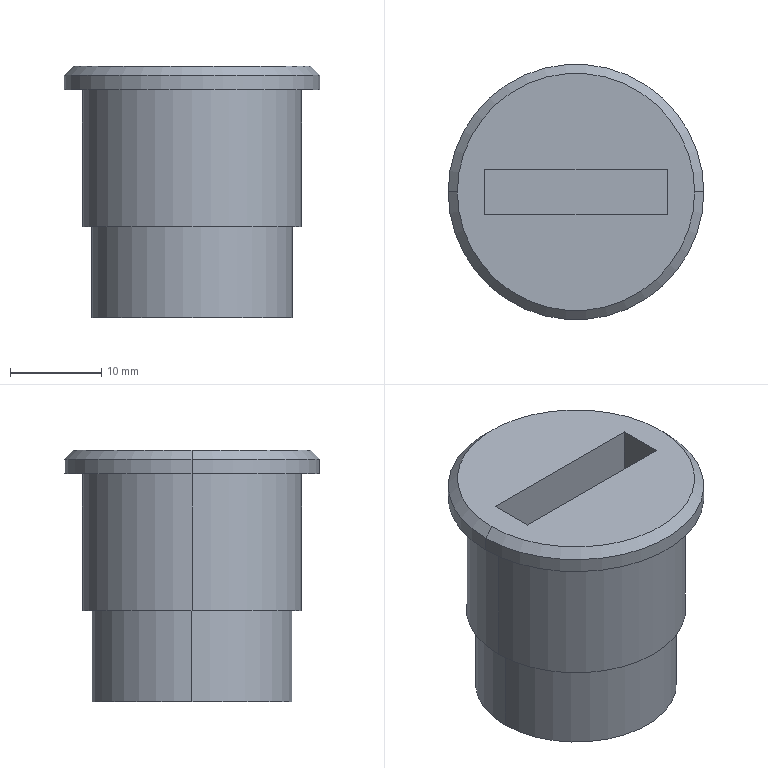Part | STEP file | USB port | 1 solid | 17 faces | box 28 x 28 x 27.6 mm | volume 11145 mm3 | plane 9 | cylinder 6 | cone 2 | commonest cylinder face diameters 22 x2 24 x2 28 x2
STEP:
#1=CARTESIAN_POINT('',(0.,0.,0.));
#2=DIRECTION('',(0.,0.,1.));
#3=DIRECTION('',(1.,0.,0.));
#4=AXIS2_PLACEMENT_3D('',#1,#2,#3);
#5=CARTESIAN_POINT('',(13.,0.,17.6));
#6=VERTEX_POINT('',#5);
#7=CARTESIAN_POINT('',(-13.,0.,17.6));
#8=VERTEX_POINT('',#7);
#9=CARTESIAN_POINT('',(0.,0.,17.6));
#10=DIRECTION('',(0.,0.,1.));
#11=DIRECTION('',(1.,0.,0.));
#12=AXIS2_PLACEMENT_3D('',#9,#10,#11);
#13=CIRCLE('',#12,13.);
#14=CARTESIAN_POINT('',(0.,0.,17.6));
#15=DIRECTION('',(0.,0.,-1.));
#16=DIRECTION('',(-1.,0.,0.));
#17=AXIS2_PLACEMENT_3D('',#14,#15,#16);
#18=CONICAL_SURFACE('',#17,13.,0.7854);
#19=CARTESIAN_POINT('',(3.142,0.));
#20=DIRECTION('',(-1.,0.));
#21=VECTOR('',#20,1.);
#22=LINE('',#19,#21);
#23=(GEOMETRIC_REPRESENTATION_CONTEXT(2)PARAMETRIC_REPRESENTATION_CONTEXT()REPRESENTATION_CONTEXT('',''));
#24=DEFINITIONAL_REPRESENTATION('',(#22),#23);
#25=PCURVE('',#18,#24);
#26=CARTESIAN_POINT('',(0.,0.,17.6));
#27=DIRECTION('',(0.,0.,1.));
#28=DIRECTION('',(1.,0.,0.));
#29=AXIS2_PLACEMENT_3D('',#26,#27,#28);
#30=PLANE('',#29);
#31=CARTESIAN_POINT('',(0.,0.));
#32=DIRECTION('',(1.,0.));
#33=AXIS2_PLACEMENT_2D('',#31,#32);
#34=CIRCLE('',#33,13.);
#35=(GEOMETRIC_REPRESENTATION_CONTEXT(2)PARAMETRIC_REPRESENTATION_CONTEXT()REPRESENTATION_CONTEXT('',''));
#36=DEFINITIONAL_REPRESENTATION('',(#34),#35);
#37=PCURVE('',#30,#36);
#38=SURFACE_CURVE('',#13,(#25,#37),.PCURVE_S1.);
#39=EDGE_CURVE('',#6,#8,#38,.T.);
#40=ORIENTED_EDGE('',*,*,#39,.F.);
#41=CARTESIAN_POINT('',(14.,0.,16.6));
#42=VERTEX_POINT('',#41);
#43=CARTESIAN_POINT('',(13.,0.,17.6));
#44=DIRECTION('',(0.7071,0.,-0.7071));
#45=VECTOR('',#44,1.);
#46=LINE('',#43,#45);
#47=CARTESIAN_POINT('',(3.142,0.));
#48=DIRECTION('',(0.,1.));
#49=VECTOR('',#48,1.);
#50=LINE('',#47,#49);
#51=(GEOMETRIC_REPRESENTATION_CONTEXT(2)PARAMETRIC_REPRESENTATION_CONTEXT()REPRESENTATION_CONTEXT('',''));
#52=DEFINITIONAL_REPRESENTATION('',(#50),#51);
#53=PCURVE('',#18,#52);
#54=CARTESIAN_POINT('',(0.,0.,17.6));
#55=DIRECTION('',(0.,0.,-1.));
#56=DIRECTION('',(-1.,0.,0.));
#57=AXIS2_PLACEMENT_3D('',#54,#55,#56);
#58=CONICAL_SURFACE('',#57,13.,0.7854);
#59=CARTESIAN_POINT('',(3.142,0.));
#60=DIRECTION('',(0.,1.));
#61=VECTOR('',#60,1.);
#62=LINE('',#59,#61);
#63=(GEOMETRIC_REPRESENTATION_CONTEXT(2)PARAMETRIC_REPRESENTATION_CONTEXT()REPRESENTATION_CONTEXT('',''));
#64=DEFINITIONAL_REPRESENTATION('',(#62),#63);
#65=PCURVE('',#58,#64);
#66=SURFACE_CURVE('',#46,(#53,#65),.PCURVE_S1.);
#67=EDGE_CURVE('',#6,#42,#66,.T.);
#68=ORIENTED_EDGE('',*,*,#67,.T.);
#69=CARTESIAN_POINT('',(-14.,0.,16.6));
#70=VERTEX_POINT('',#69);
#71=CARTESIAN_POINT('',(0.,0.,16.6));
#72=DIRECTION('',(0.,0.,-1.));
#73=DIRECTION('',(1.,0.,0.));
#74=AXIS2_PLACEMENT_3D('',#71,#72,#73);
#75=CIRCLE('',#74,14.);
#76=CARTESIAN_POINT('',(-3.142,1.));
#77=DIRECTION('',(1.,0.));
#78=VECTOR('',#77,1.);
#79=LINE('',#76,#78);
#80=(GEOMETRIC_REPRESENTATION_CONTEXT(2)PARAMETRIC_REPRESENTATION_CONTEXT()REPRESENTATION_CONTEXT('',''));
#81=DEFINITIONAL_REPRESENTATION('',(#79),#80);
#82=PCURVE('',#18,#81);
#83=CARTESIAN_POINT('',(0.,0.,17.6));
#84=DIRECTION('',(0.,0.,-1.));
#85=DIRECTION('',(-1.,0.,0.));
#86=AXIS2_PLACEMENT_3D('',#83,#84,#85);
#87=CYLINDRICAL_SURFACE('',#86,14.);
#88=CARTESIAN_POINT('',(-3.142,1.));
#89=DIRECTION('',(1.,0.));
#90=VECTOR('',#89,1.);
#91=LINE('',#88,#90);
#92=(GEOMETRIC_REPRESENTATION_CONTEXT(2)PARAMETRIC_REPRESENTATION_CONTEXT()REPRESENTATION_CONTEXT('',''));
#93=DEFINITIONAL_REPRESENTATION('',(#91),#92);
#94=PCURVE('',#87,#93);
#95=SURFACE_CURVE('',#75,(#82,#94),.PCURVE_S1.);
#96=EDGE_CURVE('',#70,#42,#95,.T.);
#97=ORIENTED_EDGE('',*,*,#96,.F.);
#98=CARTESIAN_POINT('',(-13.,0.,17.6));
#99=DIRECTION('',(-0.7071,0.,-0.7071));
#100=VECTOR('',#99,1.);
#101=LINE('',#98,#100);
#102=CARTESIAN_POINT('',(0.,0.));
#103=DIRECTION('',(0.,1.));
#104=VECTOR('',#103,1.);
#105=LINE('',#102,#104);
#106=(GEOMETRIC_REPRESENTATION_CONTEXT(2)PARAMETRIC_REPRESENTATION_CONTEXT()REPRESENTATION_CONTEXT('',''));
#107=DEFINITIONAL_REPRESENTATION('',(#105),#106);
#108=PCURVE('',#18,#107);
#109=CARTESIAN_POINT('',(6.283,0.));
#110=DIRECTION('',(0.,1.));
#111=VECTOR('',#110,1.);
#112=LINE('',#109,#111);
#113=(GEOMETRIC_REPRESENTATION_CONTEXT(2)PARAMETRIC_REPRESENTATION_CONTEXT()REPRESENTATION_CONTEXT('',''));
#114=DEFINITIONAL_REPRESENTATION('',(#112),#113);
#115=PCURVE('',#58,#114);
#116=SURFACE_CURVE('',#101,(#108,#115),.PCURVE_S1.);
#117=EDGE_CURVE('',#8,#70,#116,.T.);
#118=ORIENTED_EDGE('',*,*,#117,.F.);
#119=EDGE_LOOP('',(#40,#68,#97,#118));
#120=FACE_BOUND('',#119,.T.);
#121=ADVANCED_FACE('',(#120),#18,.T.);
#122=CARTESIAN_POINT('',(-11.,0.,-10.));
#123=VERTEX_POINT('',#122);
#124=CARTESIAN_POINT('',(11.,0.,-10.));
#125=VERTEX_POINT('',#124);
#126=CARTESIAN_POINT('',(0.,0.,-10.));
#127=DIRECTION('',(0.,0.,-1.));
#128=DIRECTION('',(-1.,0.,0.));
#129=AXIS2_PLACEMENT_3D('',#126,#127,#128);
#130=CIRCLE('',#129,11.);
#131=CARTESIAN_POINT('',(0.,0.,-10.));
#132=DIRECTION('',(0.,0.,1.));
#133=DIRECTION('',(1.,0.,0.));
#134=AXIS2_PLACEMENT_3D('',#131,#132,#133);
#135=CYLINDRICAL_SURFACE('',#134,11.);
#136=CARTESIAN_POINT('',(3.142,0.));
#137=DIRECTION('',(-1.,0.));
#138=VECTOR('',#137,1.);
#139=LINE('',#136,#138);
#140=(GEOMETRIC_REPRESENTATION_CONTEXT(2)PARAMETRIC_REPRESENTATION_CONTEXT()REPRESENTATION_CONTEXT('',''));
#141=DEFINITIONAL_REPRESENTATION('',(#139),#140);
#142=PCURVE('',#135,#141);
#143=CARTESIAN_POINT('',(0.,0.,-10.));
#144=DIRECTION('',(0.,0.,-1.));
#145=DIRECTION('',(-1.,0.,0.));
#146=AXIS2_PLACEMENT_3D('',#143,#144,#145);
#147=PLANE('',#146);
#148=CARTESIAN_POINT('',(0.,0.));
#149=DIRECTION('',(1.,0.));
#150=AXIS2_PLACEMENT_2D('',#148,#149);
#151=CIRCLE('',#150,11.);
#152=(GEOMETRIC_REPRESENTATION_CONTEXT(2)PARAMETRIC_REPRESENTATION_CONTEXT()REPRESENTATION_CONTEXT('',''));
#153=DEFINITIONAL_REPRESENTATION('',(#151),#152);
#154=PCURVE('',#147,#153);
#155=SURFACE_CURVE('',#130,(#142,#154),.PCURVE_S1.);
#156=EDGE_CURVE('',#123,#125,#155,.T.);
#157=ORIENTED_EDGE('',*,*,#156,.F.);
#158=CARTESIAN_POINT('',(-11.,0.,0.));
#159=VERTEX_POINT('',#158);
#160=CARTESIAN_POINT('',(-11.,0.,-10.));
#161=DIRECTION('',(0.,0.,1.));
#162=VECTOR('',#161,1.);
#163=LINE('',#160,#162);
#164=CARTESIAN_POINT('',(3.142,0.));
#165=DIRECTION('',(0.,1.));
#166=VECTOR('',#165,1.);
#167=LINE('',#164,#166);
#168=(GEOMETRIC_REPRESENTATION_CONTEXT(2)PARAMETRIC_REPRESENTATION_CONTEXT()REPRESENTATION_CONTEXT('',''));
#169=DEFINITIONAL_REPRESENTATION('',(#167),#168);
#170=PCURVE('',#135,#169);
#171=CARTESIAN_POINT('',(0.,0.,-10.));
#172=DIRECTION('',(0.,0.,1.));
#173=DIRECTION('',(1.,0.,0.));
#174=AXIS2_PLACEMENT_3D('',#171,#172,#173);
#175=CYLINDRICAL_SURFACE('',#174,11.);
#176=CARTESIAN_POINT('',(3.142,0.));
#177=DIRECTION('',(0.,1.));
#178=VECTOR('',#177,1.);
#179=LINE('',#176,#178);
#180=(GEOMETRIC_REPRESENTATION_CONTEXT(2)PARAMETRIC_REPRESENTATION_CONTEXT()REPRESENTATION_CONTEXT('',''));
#181=DEFINITIONAL_REPRESENTATION('',(#179),#180);
#182=PCURVE('',#175,#181);
#183=SURFACE_CURVE('',#163,(#170,#182),.PCURVE_S1.);
#184=EDGE_CURVE('',#123,#159,#183,.T.);
#185=ORIENTED_EDGE('',*,*,#184,.T.);
#186=CARTESIAN_POINT('',(11.,0.,0.));
#187=VERTEX_POINT('',#186);
#188=CARTESIAN_POINT('',(0.,0.,0.));
#189=DIRECTION('',(0.,0.,-1.));
#190=DIRECTION('',(-1.,0.,0.));
#191=AXIS2_PLACEMENT_3D('',#188,#189,#190);
#192=CIRCLE('',#191,11.);
#193=CARTESIAN_POINT('',(3.142,10.));
#194=DIRECTION('',(-1.,0.));
#195=VECTOR('',#194,1.);
#196=LINE('',#193,#195);
#197=(GEOMETRIC_REPRESENTATION_CONTEXT(2)PARAMETRIC_REPRESENTATION_CONTEXT()REPRESENTATION_CONTEXT('',''));
#198=DEFINITIONAL_REPRESENTATION('',(#196),#197);
#199=PCURVE('',#135,#198);
#200=CARTESIAN_POINT('',(0.,0.,0.));
#201=DIRECTION('',(0.,0.,1.));
#202=DIRECTION('',(1.,0.,0.));
#203=AXIS2_PLACEMENT_3D('',#200,#201,#202);
#204=PLANE('',#203);
#205=CARTESIAN_POINT('',(-11.,0.));
#206=CARTESIAN_POINT('',(-11.,19.053));
#207=CARTESIAN_POINT('',(5.5,9.526));
#208=CARTESIAN_POINT('',(22.,0.));
#209=CARTESIAN_POINT('',(5.5,-9.526));
#210=CARTESIAN_POINT('',(-11.,-19.053));
#211=CARTESIAN_POINT('',(-11.,0.));
#212=(BOUNDED_CURVE()B_SPLINE_CURVE(2,(#205,#206,#207,#208,#209,#210,#211),.UNSPECIFIED.,.T.,.F.)B_SPLINE_CURVE_WITH_KNOTS((1,2,2,2,2,1),(-2.094,0.,2.094,4.189,6.283,8.378),.UNSPECIFIED.)CURVE()GEOMETRIC_REPRESENTATION_ITEM()RATIONAL_B_SPLINE_CURVE((1.,0.5,1.,0.5,1.,0.5,1.))REPRESENTATION_ITEM(''));
#213=(GEOMETRIC_REPRESENTATION_CONTEXT(2)PARAMETRIC_REPRESENTATION_CONTEXT()REPRESENTATION_CONTEXT('',''));
#214=DEFINITIONAL_REPRESENTATION('',(#212),#213);
#215=PCURVE('',#204,#214);
#216=SURFACE_CURVE('',#192,(#199,#215),.PCURVE_S1.);
#217=EDGE_CURVE('',#159,#187,#216,.T.);
#218=ORIENTED_EDGE('',*,*,#217,.T.);
#219=CARTESIAN_POINT('',(11.,0.,-10.));
#220=DIRECTION('',(0.,0.,1.));
#221=VECTOR('',#220,1.);
#222=LINE('',#219,#221);
#223=CARTESIAN_POINT('',(0.,0.));
#224=DIRECTION('',(0.,1.));
#225=VECTOR('',#224,1.);
#226=LINE('',#223,#225);
#227=(GEOMETRIC_REPRESENTATION_CONTEXT(2)PARAMETRIC_REPRESENTATION_CONTEXT()REPRESENTATION_CONTEXT('',''));
#228=DEFINITIONAL_REPRESENTATION('',(#226),#227);
#229=PCURVE('',#135,#228);
#230=CARTESIAN_POINT('',(6.283,0.));
#231=DIRECTION('',(0.,1.));
#232=VECTOR('',#231,1.);
#233=LINE('',#230,#232);
#234=(GEOMETRIC_REPRESENTATION_CONTEXT(2)PARAMETRIC_REPRESENTATION_CONTEXT()REPRESENTATION_CONTEXT('',''));
#235=DEFINITIONAL_REPRESENTATION('',(#233),#234);
#236=PCURVE('',#175,#235);
#237=SURFACE_CURVE('',#222,(#229,#236),.PCURVE_S1.);
#238=EDGE_CURVE('',#125,#187,#237,.T.);
#239=ORIENTED_EDGE('',*,*,#238,.F.);
#240=EDGE_LOOP('',(#157,#185,#218,#239));
#241=FACE_BOUND('',#240,.T.);
#242=ADVANCED_FACE('',(#241),#135,.T.);
#243=ORIENTED_EDGE('',*,*,#96,.T.);
#244=CARTESIAN_POINT('',(14.,0.,15.));
#245=VERTEX_POINT('',#244);
#246=CARTESIAN_POINT('',(14.,0.,17.6));
#247=DIRECTION('',(0.,0.,-1.));
#248=VECTOR('',#247,1.);
#249=LINE('',#246,#248);
#250=CARTESIAN_POINT('',(3.142,0.));
#251=DIRECTION('',(0.,1.));
#252=VECTOR('',#251,1.);
#253=LINE('',#250,#252);
#254=(GEOMETRIC_REPRESENTATION_CONTEXT(2)PARAMETRIC_REPRESENTATION_CONTEXT()REPRESENTATION_CONTEXT('',''));
#255=DEFINITIONAL_REPRESENTATION('',(#253),#254);
#256=PCURVE('',#87,#255);
#257=CARTESIAN_POINT('',(0.,0.,17.6));
#258=DIRECTION('',(0.,0.,-1.));
#259=DIRECTION('',(-1.,0.,0.));
#260=AXIS2_PLACEMENT_3D('',#257,#258,#259);
#261=CYLINDRICAL_SURFACE('',#260,14.);
#262=CARTESIAN_POINT('',(3.142,0.));
#263=DIRECTION('',(0.,1.));
#264=VECTOR('',#263,1.);
#265=LINE('',#262,#264);
#266=(GEOMETRIC_REPRESENTATION_CONTEXT(2)PARAMETRIC_REPRESENTATION_CONTEXT()REPRESENTATION_CONTEXT('',''));
#267=DEFINITIONAL_REPRESENTATION('',(#265),#266);
#268=PCURVE('',#261,#267);
#269=SURFACE_CURVE('',#249,(#256,#268),.PCURVE_S1.);
#270=EDGE_CURVE('',#42,#245,#269,.T.);
#271=ORIENTED_EDGE('',*,*,#270,.T.);
#272=CARTESIAN_POINT('',(-14.,0.,15.));
#273=VERTEX_POINT('',#272);
#274=CARTESIAN_POINT('',(0.,0.,15.));
#275=DIRECTION('',(0.,0.,1.));
#276=DIRECTION('',(1.,0.,0.));
#277=AXIS2_PLACEMENT_3D('',#274,#275,#276);
#278=CIRCLE('',#277,14.);
#279=CARTESIAN_POINT('',(3.142,2.6));
#280=DIRECTION('',(-1.,0.));
#281=VECTOR('',#280,1.);
#282=LINE('',#279,#281);
#283=(GEOMETRIC_REPRESENTATION_CONTEXT(2)PARAMETRIC_REPRESENTATION_CONTEXT()REPRESENTATION_CONTEXT('',''));
#284=DEFINITIONAL_REPRESENTATION('',(#282),#283);
#285=PCURVE('',#87,#284);
#286=CARTESIAN_POINT('',(0.,0.,15.));
#287=DIRECTION('',(0.,0.,1.));
#288=DIRECTION('',(1.,0.,0.));
#289=AXIS2_PLACEMENT_3D('',#286,#287,#288);
#290=PLANE('',#289);
#291=CARTESIAN_POINT('',(0.,0.));
#292=DIRECTION('',(1.,0.));
#293=AXIS2_PLACEMENT_2D('',#291,#292);
#294=CIRCLE('',#293,14.);
#295=(GEOMETRIC_REPRESENTATION_CONTEXT(2)PARAMETRIC_REPRESENTATION_CONTEXT()REPRESENTATION_CONTEXT('',''));
#296=DEFINITIONAL_REPRESENTATION('',(#294),#295);
#297=PCURVE('',#290,#296);
#298=SURFACE_CURVE('',#278,(#285,#297),.PCURVE_S1.);
#299=EDGE_CURVE('',#245,#273,#298,.T.);
#300=ORIENTED_EDGE('',*,*,#299,.T.);
#301=CARTESIAN_POINT('',(-14.,0.,17.6));
#302=DIRECTION('',(0.,0.,-1.));
#303=VECTOR('',#302,1.);
#304=LINE('',#301,#303);
#305=CARTESIAN_POINT('',(0.,0.));
#306=DIRECTION('',(0.,1.));
#307=VECTOR('',#306,1.);
#308=LINE('',#305,#307);
#309=(GEOMETRIC_REPRESENTATION_CONTEXT(2)PARAMETRIC_REPRESENTATION_CONTEXT()REPRESENTATION_CONTEXT('',''));
#310=DEFINITIONAL_REPRESENTATION('',(#308),#309);
#311=PCURVE('',#87,#310);
#312=CARTESIAN_POINT('',(6.283,0.));
#313=DIRECTION('',(0.,1.));
#314=VECTOR('',#313,1.);
#315=LINE('',#312,#314);
#316=(GEOMETRIC_REPRESENTATION_CONTEXT(2)PARAMETRIC_REPRESENTATION_CONTEXT()REPRESENTATION_CONTEXT('',''));
#317=DEFINITIONAL_REPRESENTATION('',(#315),#316);
#318=PCURVE('',#261,#317);
#319=SURFACE_CURVE('',#304,(#311,#318),.PCURVE_S1.);
#320=EDGE_CURVE('',#70,#273,#319,.T.);
#321=ORIENTED_EDGE('',*,*,#320,.F.);
#322=EDGE_LOOP('',(#243,#271,#300,#321));
#323=FACE_BOUND('',#322,.T.);
#324=ADVANCED_FACE('',(#323),#87,.T.);
#325=CARTESIAN_POINT('',(12.,0.,15.));
#326=VERTEX_POINT('',#325);
#327=CARTESIAN_POINT('',(-12.,0.,15.));
#328=VERTEX_POINT('',#327);
#329=CARTESIAN_POINT('',(0.,0.,15.));
#330=DIRECTION('',(0.,0.,1.));
#331=DIRECTION('',(1.,0.,0.));
#332=AXIS2_PLACEMENT_3D('',#329,#330,#331);
#333=CIRCLE('',#332,12.);
#334=CARTESIAN_POINT('',(0.,0.,15.));
#335=DIRECTION('',(0.,0.,-1.));
#336=DIRECTION('',(-1.,0.,0.));
#337=AXIS2_PLACEMENT_3D('',#334,#335,#336);
#338=CYLINDRICAL_SURFACE('',#337,12.);
#339=CARTESIAN_POINT('',(3.142,0.));
#340=DIRECTION('',(-1.,0.));
#341=VECTOR('',#340,1.);
#342=LINE('',#339,#341);
#343=(GEOMETRIC_REPRESENTATION_CONTEXT(2)PARAMETRIC_REPRESENTATION_CONTEXT()REPRESENTATION_CONTEXT('',''));
#344=DEFINITIONAL_REPRESENTATION('',(#342),#343);
#345=PCURVE('',#338,#344);
#346=CARTESIAN_POINT('',(0.,0.));
#347=DIRECTION('',(1.,0.));
#348=AXIS2_PLACEMENT_2D('',#346,#347);
#349=CIRCLE('',#348,12.);
#350=(GEOMETRIC_REPRESENTATION_CONTEXT(2)PARAMETRIC_REPRESENTATION_CONTEXT()REPRESENTATION_CONTEXT('',''));
#351=DEFINITIONAL_REPRESENTATION('',(#349),#350);
#352=PCURVE('',#290,#351);
#353=SURFACE_CURVE('',#333,(#345,#352),.PCURVE_S1.);
#354=EDGE_CURVE('',#326,#328,#353,.T.);
#355=ORIENTED_EDGE('',*,*,#354,.F.);
#356=CARTESIAN_POINT('',(12.,0.,0.));
#357=VERTEX_POINT('',#356);
#358=CARTESIAN_POINT('',(12.,0.,15.));
#359=DIRECTION('',(0.,0.,-1.));
#360=VECTOR('',#359,1.);
#361=LINE('',#358,#360);
#362=CARTESIAN_POINT('',(3.142,0.));
#363=DIRECTION('',(0.,1.));
#364=VECTOR('',#363,1.);
#365=LINE('',#362,#364);
#366=(GEOMETRIC_REPRESENTATION_CONTEXT(2)PARAMETRIC_REPRESENTATION_CONTEXT()REPRESENTATION_CONTEXT('',''));
#367=DEFINITIONAL_REPRESENTATION('',(#365),#366);
#368=PCURVE('',#338,#367);
#369=CARTESIAN_POINT('',(0.,0.,15.));
#370=DIRECTION('',(0.,0.,-1.));
#371=DIRECTION('',(-1.,0.,0.));
#372=AXIS2_PLACEMENT_3D('',#369,#370,#371);
#373=CYLINDRICAL_SURFACE('',#372,12.);
#374=CARTESIAN_POINT('',(3.142,0.));
#375=DIRECTION('',(0.,1.));
#376=VECTOR('',#375,1.);
#377=LINE('',#374,#376);
#378=(GEOMETRIC_REPRESENTATION_CONTEXT(2)PARAMETRIC_REPRESENTATION_CONTEXT()REPRESENTATION_CONTEXT('',''));
#379=DEFINITIONAL_REPRESENTATION('',(#377),#378);
#380=PCURVE('',#373,#379);
#381=SURFACE_CURVE('',#361,(#368,#380),.PCURVE_S1.);
#382=EDGE_CURVE('',#326,#357,#381,.T.);
#383=ORIENTED_EDGE('',*,*,#382,.T.);
#384=CARTESIAN_POINT('',(-12.,0.,0.));
#385=VERTEX_POINT('',#384);
#386=CARTESIAN_POINT('',(0.,0.,0.));
#387=DIRECTION('',(0.,0.,1.));
#388=DIRECTION('',(1.,0.,0.));
#389=AXIS2_PLACEMENT_3D('',#386,#387,#388);
#390=CIRCLE('',#389,12.);
#391=CARTESIAN_POINT('',(3.142,15.));
#392=DIRECTION('',(-1.,0.));
#393=VECTOR('',#392,1.);
#394=LINE('',#391,#393);
#395=(GEOMETRIC_REPRESENTATION_CONTEXT(2)PARAMETRIC_REPRESENTATION_CONTEXT()REPRESENTATION_CONTEXT('',''));
#396=DEFINITIONAL_REPRESENTATION('',(#394),#395);
#397=PCURVE('',#338,#396);
#398=CARTESIAN_POINT('',(0.,0.));
#399=DIRECTION('',(1.,0.));
#400=AXIS2_PLACEMENT_2D('',#398,#399);
#401=CIRCLE('',#400,12.);
#402=(GEOMETRIC_REPRESENTATION_CONTEXT(2)PARAMETRIC_REPRESENTATION_CONTEXT()REPRESENTATION_CONTEXT('',''));
#403=DEFINITIONAL_REPRESENTATION('',(#401),#402);
#404=PCURVE('',#204,#403);
#405=SURFACE_CURVE('',#390,(#397,#404),.PCURVE_S1.);
#406=EDGE_CURVE('',#357,#385,#405,.T.);
#407=ORIENTED_EDGE('',*,*,#406,.T.);
#408=CARTESIAN_POINT('',(-12.,0.,15.));
#409=DIRECTION('',(0.,0.,-1.));
#410=VECTOR('',#409,1.);
#411=LINE('',#408,#410);
#412=CARTESIAN_POINT('',(0.,0.));
#413=DIRECTION('',(0.,1.));
#414=VECTOR('',#413,1.);
#415=LINE('',#412,#414);
#416=(GEOMETRIC_REPRESENTATION_CONTEXT(2)PARAMETRIC_REPRESENTATION_CONTEXT()REPRESENTATION_CONTEXT('',''));
#417=DEFINITIONAL_REPRESENTATION('',(#415),#416);
#418=PCURVE('',#338,#417);
#419=CARTESIAN_POINT('',(6.283,0.));
#420=DIRECTION('',(0.,1.));
#421=VECTOR('',#420,1.);
#422=LINE('',#419,#421);
#423=(GEOMETRIC_REPRESENTATION_CONTEXT(2)PARAMETRIC_REPRESENTATION_CONTEXT()REPRESENTATION_CONTEXT('',''));
#424=DEFINITIONAL_REPRESENTATION('',(#422),#423);
#425=PCURVE('',#373,#424);
#426=SURFACE_CURVE('',#411,(#418,#425),.PCURVE_S1.);
#427=EDGE_CURVE('',#328,#385,#426,.T.);
#428=ORIENTED_EDGE('',*,*,#427,.F.);
#429=EDGE_LOOP('',(#355,#383,#407,#428));
#430=FACE_BOUND('',#429,.T.);
#431=ADVANCED_FACE('',(#430),#338,.T.);
#432=ORIENTED_EDGE('',*,*,#382,.F.);
#433=CARTESIAN_POINT('',(0.,0.,15.));
#434=DIRECTION('',(0.,0.,1.));
#435=DIRECTION('',(1.,0.,0.));
#436=AXIS2_PLACEMENT_3D('',#433,#434,#435);
#437=CIRCLE('',#436,12.);
#438=CARTESIAN_POINT('',(9.425,0.));
#439=DIRECTION('',(-1.,0.));
#440=VECTOR('',#439,1.);
#441=LINE('',#438,#440);
#442=(GEOMETRIC_REPRESENTATION_CONTEXT(2)PARAMETRIC_REPRESENTATION_CONTEXT()REPRESENTATION_CONTEXT('',''));
#443=DEFINITIONAL_REPRESENTATION('',(#441),#442);
#444=PCURVE('',#373,#443);
#445=CARTESIAN_POINT('',(0.,0.));
#446=DIRECTION('',(1.,0.));
#447=AXIS2_PLACEMENT_2D('',#445,#446);
#448=CIRCLE('',#447,12.);
#449=(GEOMETRIC_REPRESENTATION_CONTEXT(2)PARAMETRIC_REPRESENTATION_CONTEXT()REPRESENTATION_CONTEXT('',''));
#450=DEFINITIONAL_REPRESENTATION('',(#448),#449);
#451=PCURVE('',#290,#450);
#452=SURFACE_CURVE('',#437,(#444,#451),.PCURVE_S1.);
#453=EDGE_CURVE('',#328,#326,#452,.T.);
#454=ORIENTED_EDGE('',*,*,#453,.F.);
#455=ORIENTED_EDGE('',*,*,#427,.T.);
#456=CARTESIAN_POINT('',(0.,0.,0.));
#457=DIRECTION('',(0.,0.,1.));
#458=DIRECTION('',(1.,0.,0.));
#459=AXIS2_PLACEMENT_3D('',#456,#457,#458);
#460=CIRCLE('',#459,12.);
#461=CARTESIAN_POINT('',(9.425,15.));
#462=DIRECTION('',(-1.,0.));
#463=VECTOR('',#462,1.);
#464=LINE('',#461,#463);
#465=(GEOMETRIC_REPRESENTATION_CONTEXT(2)PARAMETRIC_REPRESENTATION_CONTEXT()REPRESENTATION_CONTEXT('',''));
#466=DEFINITIONAL_REPRESENTATION('',(#464),#465);
#467=PCURVE('',#373,#466);
#468=CARTESIAN_POINT('',(0.,0.));
#469=DIRECTION('',(1.,0.));
#470=AXIS2_PLACEMENT_2D('',#468,#469);
#471=CIRCLE('',#470,12.);
#472=(GEOMETRIC_REPRESENTATION_CONTEXT(2)PARAMETRIC_REPRESENTATION_CONTEXT()REPRESENTATION_CONTEXT('',''));
#473=DEFINITIONAL_REPRESENTATION('',(#471),#472);
#474=PCURVE('',#204,#473);
#475=SURFACE_CURVE('',#460,(#467,#474),.PCURVE_S1.);
#476=EDGE_CURVE('',#385,#357,#475,.T.);
#477=ORIENTED_EDGE('',*,*,#476,.T.);
#478=EDGE_LOOP('',(#432,#454,#455,#477));
#479=FACE_BOUND('',#478,.T.);
#480=ADVANCED_FACE('',(#479),#373,.T.);
#481=CARTESIAN_POINT('',(0.,0.,0.));
#482=DIRECTION('',(0.,0.,-1.));
#483=DIRECTION('',(-1.,0.,0.));
#484=AXIS2_PLACEMENT_3D('',#481,#482,#483);
#485=CIRCLE('',#484,11.);
#486=CARTESIAN_POINT('',(-11.,0.));
#487=CARTESIAN_POINT('',(-11.,19.053));
#488=CARTESIAN_POINT('',(5.5,9.526));
#489=CARTESIAN_POINT('',(22.,0.));
#490=CARTESIAN_POINT('',(5.5,-9.526));
#491=CARTESIAN_POINT('',(-11.,-19.053));
#492=CARTESIAN_POINT('',(-11.,0.));
#493=(BOUNDED_CURVE()B_SPLINE_CURVE(2,(#486,#487,#488,#489,#490,#491,#492),.UNSPECIFIED.,.T.,.F.)B_SPLINE_CURVE_WITH_KNOTS((1,2,2,2,2,1),(-2.094,0.,2.094,4.189,6.283,8.378),.UNSPECIFIED.)CURVE()GEOMETRIC_REPRESENTATION_ITEM()RATIONAL_B_SPLINE_CURVE((1.,0.5,1.,0.5,1.,0.5,1.))REPRESENTATION_ITEM(''));
#494=(GEOMETRIC_REPRESENTATION_CONTEXT(2)PARAMETRIC_REPRESENTATION_CONTEXT()REPRESENTATION_CONTEXT('',''));
#495=DEFINITIONAL_REPRESENTATION('',(#493),#494);
#496=PCURVE('',#204,#495);
#497=CARTESIAN_POINT('',(9.425,10.));
#498=DIRECTION('',(-1.,0.));
#499=VECTOR('',#498,1.);
#500=LINE('',#497,#499);
#501=(GEOMETRIC_REPRESENTATION_CONTEXT(2)PARAMETRIC_REPRESENTATION_CONTEXT()REPRESENTATION_CONTEXT('',''));
#502=DEFINITIONAL_REPRESENTATION('',(#500),#501);
#503=PCURVE('',#175,#502);
#504=SURFACE_CURVE('',#485,(#496,#503),.PCURVE_S1.);
#505=EDGE_CURVE('',#187,#159,#504,.T.);
#506=ORIENTED_EDGE('',*,*,#505,.F.);
#507=ORIENTED_EDGE('',*,*,#217,.F.);
#508=EDGE_LOOP('',(#506,#507));
#509=FACE_BOUND('',#508,.T.);
#510=ORIENTED_EDGE('',*,*,#476,.F.);
#511=ORIENTED_EDGE('',*,*,#406,.F.);
#512=EDGE_LOOP('',(#510,#511));
#513=FACE_BOUND('',#512,.T.);
#514=ADVANCED_FACE('',(#509,#513),#204,.F.);
#515=ORIENTED_EDGE('',*,*,#270,.F.);
#516=CARTESIAN_POINT('',(0.,0.,16.6));
#517=DIRECTION('',(0.,0.,-1.));
#518=DIRECTION('',(1.,0.,0.));
#519=AXIS2_PLACEMENT_3D('',#516,#517,#518);
#520=CIRCLE('',#519,14.);
#521=CARTESIAN_POINT('',(3.142,1.));
#522=DIRECTION('',(1.,0.));
#523=VECTOR('',#522,1.);
#524=LINE('',#521,#523);
#525=(GEOMETRIC_REPRESENTATION_CONTEXT(2)PARAMETRIC_REPRESENTATION_CONTEXT()REPRESENTATION_CONTEXT('',''));
#526=DEFINITIONAL_REPRESENTATION('',(#524),#525);
#527=PCURVE('',#261,#526);
#528=CARTESIAN_POINT('',(3.142,1.));
#529=DIRECTION('',(1.,0.));
#530=VECTOR('',#529,1.);
#531=LINE('',#528,#530);
#532=(GEOMETRIC_REPRESENTATION_CONTEXT(2)PARAMETRIC_REPRESENTATION_CONTEXT()REPRESENTATION_CONTEXT('',''));
#533=DEFINITIONAL_REPRESENTATION('',(#531),#532);
#534=PCURVE('',#58,#533);
#535=SURFACE_CURVE('',#520,(#527,#534),.PCURVE_S1.);
#536=EDGE_CURVE('',#42,#70,#535,.T.);
#537=ORIENTED_EDGE('',*,*,#536,.T.);
#538=ORIENTED_EDGE('',*,*,#320,.T.);
#539=CARTESIAN_POINT('',(0.,0.,15.));
#540=DIRECTION('',(0.,0.,1.));
#541=DIRECTION('',(1.,0.,0.));
#542=AXIS2_PLACEMENT_3D('',#539,#540,#541);
#543=CIRCLE('',#542,14.);
#544=CARTESIAN_POINT('',(9.425,2.6));
#545=DIRECTION('',(-1.,0.));
#546=VECTOR('',#545,1.);
#547=LINE('',#544,#546);
#548=(GEOMETRIC_REPRESENTATION_CONTEXT(2)PARAMETRIC_REPRESENTATION_CONTEXT()REPRESENTATION_CONTEXT('',''));
#549=DEFINITIONAL_REPRESENTATION('',(#547),#548);
#550=PCURVE('',#261,#549);
#551=CARTESIAN_POINT('',(0.,0.));
#552=DIRECTION('',(1.,0.));
#553=AXIS2_PLACEMENT_2D('',#551,#552);
#554=CIRCLE('',#553,14.);
#555=(GEOMETRIC_REPRESENTATION_CONTEXT(2)PARAMETRIC_REPRESENTATION_CONTEXT()REPRESENTATION_CONTEXT('',''));
#556=DEFINITIONAL_REPRESENTATION('',(#554),#555);
#557=PCURVE('',#290,#556);
#558=SURFACE_CURVE('',#543,(#550,#557),.PCURVE_S1.);
#559=EDGE_CURVE('',#273,#245,#558,.T.);
#560=ORIENTED_EDGE('',*,*,#559,.T.);
#561=EDGE_LOOP('',(#515,#537,#538,#560));
#562=FACE_BOUND('',#561,.T.);
#563=ADVANCED_FACE('',(#562),#261,.T.);
#564=CARTESIAN_POINT('',(0.,0.,17.6));
#565=DIRECTION('',(0.,0.,1.));
#566=DIRECTION('',(1.,0.,0.));
#567=AXIS2_PLACEMENT_3D('',#564,#565,#566);
#568=CIRCLE('',#567,13.);
#569=CARTESIAN_POINT('',(0.,0.));
#570=DIRECTION('',(1.,0.));
#571=AXIS2_PLACEMENT_2D('',#569,#570);
#572=CIRCLE('',#571,13.);
#573=(GEOMETRIC_REPRESENTATION_CONTEXT(2)PARAMETRIC_REPRESENTATION_CONTEXT()REPRESENTATION_CONTEXT('',''));
#574=DEFINITIONAL_REPRESENTATION('',(#572),#573);
#575=PCURVE('',#30,#574);
#576=CARTESIAN_POINT('',(9.425,0.));
#577=DIRECTION('',(-1.,0.));
#578=VECTOR('',#577,1.);
#579=LINE('',#576,#578);
#580=(GEOMETRIC_REPRESENTATION_CONTEXT(2)PARAMETRIC_REPRESENTATION_CONTEXT()REPRESENTATION_CONTEXT('',''));
#581=DEFINITIONAL_REPRESENTATION('',(#579),#580);
#582=PCURVE('',#58,#581);
#583=SURFACE_CURVE('',#568,(#575,#582),.PCURVE_S1.);
#584=EDGE_CURVE('',#8,#6,#583,.T.);
#585=ORIENTED_EDGE('',*,*,#584,.T.);
#586=ORIENTED_EDGE('',*,*,#39,.T.);
#587=EDGE_LOOP('',(#585,#586));
#588=FACE_BOUND('',#587,.T.);
#589=CARTESIAN_POINT('',(10.,-2.5,17.6));
#590=VERTEX_POINT('',#589);
#591=CARTESIAN_POINT('',(10.,2.5,17.6));
#592=VERTEX_POINT('',#591);
#593=CARTESIAN_POINT('',(10.,2.5,17.6));
#594=DIRECTION('',(0.,1.,0.));
#595=VECTOR('',#594,1.);
#596=LINE('',#593,#595);
#597=CARTESIAN_POINT('',(10.,2.5));
#598=DIRECTION('',(0.,1.));
#599=VECTOR('',#598,1.);
#600=LINE('',#597,#599);
#601=(GEOMETRIC_REPRESENTATION_CONTEXT(2)PARAMETRIC_REPRESENTATION_CONTEXT()REPRESENTATION_CONTEXT('',''));
#602=DEFINITIONAL_REPRESENTATION('',(#600),#601);
#603=PCURVE('',#30,#602);
#604=CARTESIAN_POINT('',(10.,2.5,7.6));
#605=DIRECTION('',(1.,0.,0.));
#606=DIRECTION('',(0.,0.,-1.));
#607=AXIS2_PLACEMENT_3D('',#604,#605,#606);
#608=PLANE('',#607);
#609=CARTESIAN_POINT('',(-10.,0.));
#610=DIRECTION('',(0.,1.));
#611=VECTOR('',#610,1.);
#612=LINE('',#609,#611);
#613=(GEOMETRIC_REPRESENTATION_CONTEXT(2)PARAMETRIC_REPRESENTATION_CONTEXT()REPRESENTATION_CONTEXT('',''));
#614=DEFINITIONAL_REPRESENTATION('',(#612),#613);
#615=PCURVE('',#608,#614);
#616=SURFACE_CURVE('',#596,(#603,#615),.PCURVE_S1.);
#617=EDGE_CURVE('',#590,#592,#616,.T.);
#618=ORIENTED_EDGE('',*,*,#617,.F.);
#619=CARTESIAN_POINT('',(-10.,-2.5,17.6));
#620=VERTEX_POINT('',#619);
#621=CARTESIAN_POINT('',(-10.,-2.5,17.6));
#622=DIRECTION('',(1.,0.,0.));
#623=VECTOR('',#622,1.);
#624=LINE('',#621,#623);
#625=CARTESIAN_POINT('',(-10.,-2.5));
#626=DIRECTION('',(1.,0.));
#627=VECTOR('',#626,1.);
#628=LINE('',#625,#627);
#629=(GEOMETRIC_REPRESENTATION_CONTEXT(2)PARAMETRIC_REPRESENTATION_CONTEXT()REPRESENTATION_CONTEXT('',''));
#630=DEFINITIONAL_REPRESENTATION('',(#628),#629);
#631=PCURVE('',#30,#630);
#632=CARTESIAN_POINT('',(-10.,-2.5,7.6));
#633=DIRECTION('',(0.,-1.,0.));
#634=DIRECTION('',(0.,0.,-1.));
#635=AXIS2_PLACEMENT_3D('',#632,#633,#634);
#636=PLANE('',#635);
#637=CARTESIAN_POINT('',(-10.,0.));
#638=DIRECTION('',(0.,1.));
#639=VECTOR('',#638,1.);
#640=LINE('',#637,#639);
#641=(GEOMETRIC_REPRESENTATION_CONTEXT(2)PARAMETRIC_REPRESENTATION_CONTEXT()REPRESENTATION_CONTEXT('',''));
#642=DEFINITIONAL_REPRESENTATION('',(#640),#641);
#643=PCURVE('',#636,#642);
#644=SURFACE_CURVE('',#624,(#631,#643),.PCURVE_S1.);
#645=EDGE_CURVE('',#620,#590,#644,.T.);
#646=ORIENTED_EDGE('',*,*,#645,.F.);
#647=CARTESIAN_POINT('',(-10.,2.5,17.6));
#648=VERTEX_POINT('',#647);
#649=CARTESIAN_POINT('',(-10.,2.5,17.6));
#650=DIRECTION('',(0.,-1.,0.));
#651=VECTOR('',#650,1.);
#652=LINE('',#649,#651);
#653=CARTESIAN_POINT('',(-10.,2.5));
#654=DIRECTION('',(0.,-1.));
#655=VECTOR('',#654,1.);
#656=LINE('',#653,#655);
#657=(GEOMETRIC_REPRESENTATION_CONTEXT(2)PARAMETRIC_REPRESENTATION_CONTEXT()REPRESENTATION_CONTEXT('',''));
#658=DEFINITIONAL_REPRESENTATION('',(#656),#657);
#659=PCURVE('',#30,#658);
#660=CARTESIAN_POINT('',(-10.,2.5,7.6));
#661=DIRECTION('',(-1.,0.,0.));
#662=DIRECTION('',(0.,0.,1.));
#663=AXIS2_PLACEMENT_3D('',#660,#661,#662);
#664=PLANE('',#663);
#665=CARTESIAN_POINT('',(10.,0.));
#666=DIRECTION('',(0.,-1.));
#667=VECTOR('',#666,1.);
#668=LINE('',#665,#667);
#669=(GEOMETRIC_REPRESENTATION_CONTEXT(2)PARAMETRIC_REPRESENTATION_CONTEXT()REPRESENTATION_CONTEXT('',''));
#670=DEFINITIONAL_REPRESENTATION('',(#668),#669);
#671=PCURVE('',#664,#670);
#672=SURFACE_CURVE('',#652,(#659,#671),.PCURVE_S1.);
#673=EDGE_CURVE('',#648,#620,#672,.T.);
#674=ORIENTED_EDGE('',*,*,#673,.F.);
#675=CARTESIAN_POINT('',(-10.,2.5,17.6));
#676=DIRECTION('',(-1.,0.,0.));
#677=VECTOR('',#676,1.);
#678=LINE('',#675,#677);
#679=CARTESIAN_POINT('',(-10.,2.5));
#680=DIRECTION('',(-1.,0.));
#681=VECTOR('',#680,1.);
#682=LINE('',#679,#681);
#683=(GEOMETRIC_REPRESENTATION_CONTEXT(2)PARAMETRIC_REPRESENTATION_CONTEXT()REPRESENTATION_CONTEXT('',''));
#684=DEFINITIONAL_REPRESENTATION('',(#682),#683);
#685=PCURVE('',#30,#684);
#686=CARTESIAN_POINT('',(-10.,2.5,7.6));
#687=DIRECTION('',(0.,1.,0.));
#688=DIRECTION('',(0.,0.,1.));
#689=AXIS2_PLACEMENT_3D('',#686,#687,#688);
#690=PLANE('',#689);
#691=CARTESIAN_POINT('',(10.,0.));
#692=DIRECTION('',(0.,-1.));
#693=VECTOR('',#692,1.);
#694=LINE('',#691,#693);
#695=(GEOMETRIC_REPRESENTATION_CONTEXT(2)PARAMETRIC_REPRESENTATION_CONTEXT()REPRESENTATION_CONTEXT('',''));
#696=DEFINITIONAL_REPRESENTATION('',(#694),#695);
#697=PCURVE('',#690,#696);
#698=SURFACE_CURVE('',#678,(#685,#697),.PCURVE_S1.);
#699=EDGE_CURVE('',#592,#648,#698,.T.);
#700=ORIENTED_EDGE('',*,*,#699,.F.);
#701=EDGE_LOOP('',(#618,#646,#674,#700));
#702=FACE_BOUND('',#701,.T.);
#703=ADVANCED_FACE('',(#588,#702),#30,.T.);
#704=ORIENTED_EDGE('',*,*,#453,.T.);
#705=ORIENTED_EDGE('',*,*,#354,.T.);
#706=EDGE_LOOP('',(#704,#705));
#707=FACE_BOUND('',#706,.T.);
#708=ORIENTED_EDGE('',*,*,#559,.F.);
#709=ORIENTED_EDGE('',*,*,#299,.F.);
#710=EDGE_LOOP('',(#708,#709));
#711=FACE_BOUND('',#710,.T.);
#712=ADVANCED_FACE('',(#707,#711),#290,.F.);
#713=ORIENTED_EDGE('',*,*,#184,.F.);
#714=CARTESIAN_POINT('',(0.,0.,-10.));
#715=DIRECTION('',(0.,0.,-1.));
#716=DIRECTION('',(-1.,0.,0.));
#717=AXIS2_PLACEMENT_3D('',#714,#715,#716);
#718=CIRCLE('',#717,11.);
#719=CARTESIAN_POINT('',(9.425,0.));
#720=DIRECTION('',(-1.,0.));
#721=VECTOR('',#720,1.);
#722=LINE('',#719,#721);
#723=(GEOMETRIC_REPRESENTATION_CONTEXT(2)PARAMETRIC_REPRESENTATION_CONTEXT()REPRESENTATION_CONTEXT('',''));
#724=DEFINITIONAL_REPRESENTATION('',(#722),#723);
#725=PCURVE('',#175,#724);
#726=CARTESIAN_POINT('',(0.,0.));
#727=DIRECTION('',(1.,0.));
#728=AXIS2_PLACEMENT_2D('',#726,#727);
#729=CIRCLE('',#728,11.);
#730=(GEOMETRIC_REPRESENTATION_CONTEXT(2)PARAMETRIC_REPRESENTATION_CONTEXT()REPRESENTATION_CONTEXT('',''));
#731=DEFINITIONAL_REPRESENTATION('',(#729),#730);
#732=PCURVE('',#147,#731);
#733=SURFACE_CURVE('',#718,(#725,#732),.PCURVE_S1.);
#734=EDGE_CURVE('',#125,#123,#733,.T.);
#735=ORIENTED_EDGE('',*,*,#734,.F.);
#736=ORIENTED_EDGE('',*,*,#238,.T.);
#737=ORIENTED_EDGE('',*,*,#505,.T.);
#738=EDGE_LOOP('',(#713,#735,#736,#737));
#739=FACE_BOUND('',#738,.T.);
#740=ADVANCED_FACE('',(#739),#175,.T.);
#741=ORIENTED_EDGE('',*,*,#734,.T.);
#742=ORIENTED_EDGE('',*,*,#156,.T.);
#743=EDGE_LOOP('',(#741,#742));
#744=FACE_BOUND('',#743,.T.);
#745=ADVANCED_FACE('',(#744),#147,.T.);
#746=ORIENTED_EDGE('',*,*,#617,.T.);
#747=CARTESIAN_POINT('',(10.,2.5,7.6));
#748=VERTEX_POINT('',#747);
#749=CARTESIAN_POINT('',(10.,2.5,7.6));
#750=DIRECTION('',(0.,0.,1.));
#751=VECTOR('',#750,1.);
#752=LINE('',#749,#751);
#753=CARTESIAN_POINT('',(0.,0.));
#754=DIRECTION('',(-1.,0.));
#755=VECTOR('',#754,1.);
#756=LINE('',#753,#755);
#757=(GEOMETRIC_REPRESENTATION_CONTEXT(2)PARAMETRIC_REPRESENTATION_CONTEXT()REPRESENTATION_CONTEXT('',''));
#758=DEFINITIONAL_REPRESENTATION('',(#756),#757);
#759=PCURVE('',#608,#758);
#760=CARTESIAN_POINT('',(0.,20.));
#761=DIRECTION('',(1.,0.));
#762=VECTOR('',#761,1.);
#763=LINE('',#760,#762);
#764=(GEOMETRIC_REPRESENTATION_CONTEXT(2)PARAMETRIC_REPRESENTATION_CONTEXT()REPRESENTATION_CONTEXT('',''));
#765=DEFINITIONAL_REPRESENTATION('',(#763),#764);
#766=PCURVE('',#690,#765);
#767=SURFACE_CURVE('',#752,(#759,#766),.PCURVE_S1.);
#768=EDGE_CURVE('',#748,#592,#767,.T.);
#769=ORIENTED_EDGE('',*,*,#768,.F.);
#770=CARTESIAN_POINT('',(10.,-2.5,7.6));
#771=VERTEX_POINT('',#770);
#772=CARTESIAN_POINT('',(10.,2.5,7.6));
#773=DIRECTION('',(0.,1.,0.));
#774=VECTOR('',#773,1.);
#775=LINE('',#772,#774);
#776=CARTESIAN_POINT('',(0.,0.));
#777=DIRECTION('',(0.,1.));
#778=VECTOR('',#777,1.);
#779=LINE('',#776,#778);
#780=(GEOMETRIC_REPRESENTATION_CONTEXT(2)PARAMETRIC_REPRESENTATION_CONTEXT()REPRESENTATION_CONTEXT('',''));
#781=DEFINITIONAL_REPRESENTATION('',(#779),#780);
#782=PCURVE('',#608,#781);
#783=CARTESIAN_POINT('',(0.,0.,7.6));
#784=DIRECTION('',(0.,0.,1.));
#785=DIRECTION('',(1.,0.,0.));
#786=AXIS2_PLACEMENT_3D('',#783,#784,#785);
#787=PLANE('',#786);
#788=CARTESIAN_POINT('',(10.,2.5));
#789=DIRECTION('',(0.,1.));
#790=VECTOR('',#789,1.);
#791=LINE('',#788,#790);
#792=(GEOMETRIC_REPRESENTATION_CONTEXT(2)PARAMETRIC_REPRESENTATION_CONTEXT()REPRESENTATION_CONTEXT('',''));
#793=DEFINITIONAL_REPRESENTATION('',(#791),#792);
#794=PCURVE('',#787,#793);
#795=SURFACE_CURVE('',#775,(#782,#794),.PCURVE_S1.);
#796=EDGE_CURVE('',#771,#748,#795,.T.);
#797=ORIENTED_EDGE('',*,*,#796,.F.);
#798=CARTESIAN_POINT('',(10.,-2.5,7.6));
#799=DIRECTION('',(0.,0.,1.));
#800=VECTOR('',#799,1.);
#801=LINE('',#798,#800);
#802=CARTESIAN_POINT('',(0.,-5.));
#803=DIRECTION('',(-1.,0.));
#804=VECTOR('',#803,1.);
#805=LINE('',#802,#804);
#806=(GEOMETRIC_REPRESENTATION_CONTEXT(2)PARAMETRIC_REPRESENTATION_CONTEXT()REPRESENTATION_CONTEXT('',''));
#807=DEFINITIONAL_REPRESENTATION('',(#805),#806);
#808=PCURVE('',#608,#807);
#809=CARTESIAN_POINT('',(0.,20.));
#810=DIRECTION('',(-1.,0.));
#811=VECTOR('',#810,1.);
#812=LINE('',#809,#811);
#813=(GEOMETRIC_REPRESENTATION_CONTEXT(2)PARAMETRIC_REPRESENTATION_CONTEXT()REPRESENTATION_CONTEXT('',''));
#814=DEFINITIONAL_REPRESENTATION('',(#812),#813);
#815=PCURVE('',#636,#814);
#816=SURFACE_CURVE('',#801,(#808,#815),.PCURVE_S1.);
#817=EDGE_CURVE('',#771,#590,#816,.T.);
#818=ORIENTED_EDGE('',*,*,#817,.T.);
#819=EDGE_LOOP('',(#746,#769,#797,#818));
#820=FACE_BOUND('',#819,.T.);
#821=ADVANCED_FACE('',(#820),#608,.F.);
#822=ORIENTED_EDGE('',*,*,#645,.T.);
#823=ORIENTED_EDGE('',*,*,#817,.F.);
#824=CARTESIAN_POINT('',(-10.,-2.5,7.6));
#825=VERTEX_POINT('',#824);
#826=CARTESIAN_POINT('',(-10.,-2.5,7.6));
#827=DIRECTION('',(1.,0.,0.));
#828=VECTOR('',#827,1.);
#829=LINE('',#826,#828);
#830=CARTESIAN_POINT('',(0.,0.));
#831=DIRECTION('',(0.,1.));
#832=VECTOR('',#831,1.);
#833=LINE('',#830,#832);
#834=(GEOMETRIC_REPRESENTATION_CONTEXT(2)PARAMETRIC_REPRESENTATION_CONTEXT()REPRESENTATION_CONTEXT('',''));
#835=DEFINITIONAL_REPRESENTATION('',(#833),#834);
#836=PCURVE('',#636,#835);
#837=CARTESIAN_POINT('',(-10.,-2.5));
#838=DIRECTION('',(1.,0.));
#839=VECTOR('',#838,1.);
#840=LINE('',#837,#839);
#841=(GEOMETRIC_REPRESENTATION_CONTEXT(2)PARAMETRIC_REPRESENTATION_CONTEXT()REPRESENTATION_CONTEXT('',''));
#842=DEFINITIONAL_REPRESENTATION('',(#840),#841);
#843=PCURVE('',#787,#842);
#844=SURFACE_CURVE('',#829,(#836,#843),.PCURVE_S1.);
#845=EDGE_CURVE('',#825,#771,#844,.T.);
#846=ORIENTED_EDGE('',*,*,#845,.F.);
#847=CARTESIAN_POINT('',(-10.,-2.5,7.6));
#848=DIRECTION('',(0.,0.,1.));
#849=VECTOR('',#848,1.);
#850=LINE('',#847,#849);
#851=CARTESIAN_POINT('',(0.,0.));
#852=DIRECTION('',(-1.,0.));
#853=VECTOR('',#852,1.);
#854=LINE('',#851,#853);
#855=(GEOMETRIC_REPRESENTATION_CONTEXT(2)PARAMETRIC_REPRESENTATION_CONTEXT()REPRESENTATION_CONTEXT('',''));
#856=DEFINITIONAL_REPRESENTATION('',(#854),#855);
#857=PCURVE('',#636,#856);
#858=CARTESIAN_POINT('',(0.,-5.));
#859=DIRECTION('',(1.,0.));
#860=VECTOR('',#859,1.);
#861=LINE('',#858,#860);
#862=(GEOMETRIC_REPRESENTATION_CONTEXT(2)PARAMETRIC_REPRESENTATION_CONTEXT()REPRESENTATION_CONTEXT('',''));
#863=DEFINITIONAL_REPRESENTATION('',(#861),#862);
#864=PCURVE('',#664,#863);
#865=SURFACE_CURVE('',#850,(#857,#864),.PCURVE_S1.);
#866=EDGE_CURVE('',#825,#620,#865,.T.);
#867=ORIENTED_EDGE('',*,*,#866,.T.);
#868=EDGE_LOOP('',(#822,#823,#846,#867));
#869=FACE_BOUND('',#868,.T.);
#870=ADVANCED_FACE('',(#869),#636,.F.);
#871=ORIENTED_EDGE('',*,*,#673,.T.);
#872=ORIENTED_EDGE('',*,*,#866,.F.);
#873=CARTESIAN_POINT('',(-10.,2.5,7.6));
#874=VERTEX_POINT('',#873);
#875=CARTESIAN_POINT('',(-10.,2.5,7.6));
#876=DIRECTION('',(0.,-1.,0.));
#877=VECTOR('',#876,1.);
#878=LINE('',#875,#877);
#879=CARTESIAN_POINT('',(0.,0.));
#880=DIRECTION('',(0.,-1.));
#881=VECTOR('',#880,1.);
#882=LINE('',#879,#881);
#883=(GEOMETRIC_REPRESENTATION_CONTEXT(2)PARAMETRIC_REPRESENTATION_CONTEXT()REPRESENTATION_CONTEXT('',''));
#884=DEFINITIONAL_REPRESENTATION('',(#882),#883);
#885=PCURVE('',#664,#884);
#886=CARTESIAN_POINT('',(-10.,2.5));
#887=DIRECTION('',(0.,-1.));
#888=VECTOR('',#887,1.);
#889=LINE('',#886,#888);
#890=(GEOMETRIC_REPRESENTATION_CONTEXT(2)PARAMETRIC_REPRESENTATION_CONTEXT()REPRESENTATION_CONTEXT('',''));
#891=DEFINITIONAL_REPRESENTATION('',(#889),#890);
#892=PCURVE('',#787,#891);
#893=SURFACE_CURVE('',#878,(#885,#892),.PCURVE_S1.);
#894=EDGE_CURVE('',#874,#825,#893,.T.);
#895=ORIENTED_EDGE('',*,*,#894,.F.);
#896=CARTESIAN_POINT('',(-10.,2.5,7.6));
#897=DIRECTION('',(0.,0.,1.));
#898=VECTOR('',#897,1.);
#899=LINE('',#896,#898);
#900=CARTESIAN_POINT('',(0.,0.));
#901=DIRECTION('',(1.,0.));
#902=VECTOR('',#901,1.);
#903=LINE('',#900,#902);
#904=(GEOMETRIC_REPRESENTATION_CONTEXT(2)PARAMETRIC_REPRESENTATION_CONTEXT()REPRESENTATION_CONTEXT('',''));
#905=DEFINITIONAL_REPRESENTATION('',(#903),#904);
#906=PCURVE('',#664,#905);
#907=CARTESIAN_POINT('',(0.,0.));
#908=DIRECTION('',(1.,0.));
#909=VECTOR('',#908,1.);
#910=LINE('',#907,#909);
#911=(GEOMETRIC_REPRESENTATION_CONTEXT(2)PARAMETRIC_REPRESENTATION_CONTEXT()REPRESENTATION_CONTEXT('',''));
#912=DEFINITIONAL_REPRESENTATION('',(#910),#911);
#913=PCURVE('',#690,#912);
#914=SURFACE_CURVE('',#899,(#906,#913),.PCURVE_S1.);
#915=EDGE_CURVE('',#874,#648,#914,.T.);
#916=ORIENTED_EDGE('',*,*,#915,.T.);
#917=EDGE_LOOP('',(#871,#872,#895,#916));
#918=FACE_BOUND('',#917,.T.);
#919=ADVANCED_FACE('',(#918),#664,.F.);
#920=ORIENTED_EDGE('',*,*,#699,.T.);
#921=ORIENTED_EDGE('',*,*,#915,.F.);
#922=CARTESIAN_POINT('',(-10.,2.5,7.6));
#923=DIRECTION('',(-1.,0.,0.));
#924=VECTOR('',#923,1.);
#925=LINE('',#922,#924);
#926=CARTESIAN_POINT('',(0.,0.));
#927=DIRECTION('',(0.,-1.));
#928=VECTOR('',#927,1.);
#929=LINE('',#926,#928);
#930=(GEOMETRIC_REPRESENTATION_CONTEXT(2)PARAMETRIC_REPRESENTATION_CONTEXT()REPRESENTATION_CONTEXT('',''));
#931=DEFINITIONAL_REPRESENTATION('',(#929),#930);
#932=PCURVE('',#690,#931);
#933=CARTESIAN_POINT('',(-10.,2.5));
#934=DIRECTION('',(-1.,0.));
#935=VECTOR('',#934,1.);
#936=LINE('',#933,#935);
#937=(GEOMETRIC_REPRESENTATION_CONTEXT(2)PARAMETRIC_REPRESENTATION_CONTEXT()REPRESENTATION_CONTEXT('',''));
#938=DEFINITIONAL_REPRESENTATION('',(#936),#937);
#939=PCURVE('',#787,#938);
#940=SURFACE_CURVE('',#925,(#932,#939),.PCURVE_S1.);
#941=EDGE_CURVE('',#748,#874,#940,.T.);
#942=ORIENTED_EDGE('',*,*,#941,.F.);
#943=ORIENTED_EDGE('',*,*,#768,.T.);
#944=EDGE_LOOP('',(#920,#921,#942,#943));
#945=FACE_BOUND('',#944,.T.);
#946=ADVANCED_FACE('',(#945),#690,.F.);
#947=ORIENTED_EDGE('',*,*,#796,.T.);
#948=ORIENTED_EDGE('',*,*,#941,.T.);
#949=ORIENTED_EDGE('',*,*,#894,.T.);
#950=ORIENTED_EDGE('',*,*,#845,.T.);
#951=EDGE_LOOP('',(#947,#948,#949,#950));
#952=FACE_BOUND('',#951,.T.);
#953=ADVANCED_FACE('',(#952),#787,.T.);
#954=ORIENTED_EDGE('',*,*,#67,.F.);
#955=ORIENTED_EDGE('',*,*,#584,.F.);
#956=ORIENTED_EDGE('',*,*,#117,.T.);
#957=ORIENTED_EDGE('',*,*,#536,.F.);
#958=EDGE_LOOP('',(#954,#955,#956,#957));
#959=FACE_BOUND('',#958,.T.);
#960=ADVANCED_FACE('',(#959),#58,.T.);
#961=CLOSED_SHELL('',(#121,#242,#324,#431,#480,#514,#563,#703,#712,#740,#745,#821,#870,#919,#946,#953,#960));
#962=MANIFOLD_SOLID_BREP('',#961);
#963=(LENGTH_UNIT()NAMED_UNIT(*)SI_UNIT(.MILLI.,.METRE.));
#964=UNCERTAINTY_MEASURE_WITH_UNIT(LENGTH_MEASURE(0.0000001),#963,'','');
#965=(NAMED_UNIT(*)PLANE_ANGLE_UNIT()SI_UNIT($,.RADIAN.));
#966=(NAMED_UNIT(*)SI_UNIT($,.STERADIAN.)SOLID_ANGLE_UNIT());
#967=(GEOMETRIC_REPRESENTATION_CONTEXT(3)GLOBAL_UNCERTAINTY_ASSIGNED_CONTEXT((#964))GLOBAL_UNIT_ASSIGNED_CONTEXT((#963,#965,#966))REPRESENTATION_CONTEXT('',''));
#968=ADVANCED_BREP_SHAPE_REPRESENTATION('',(#4,#962),#967);